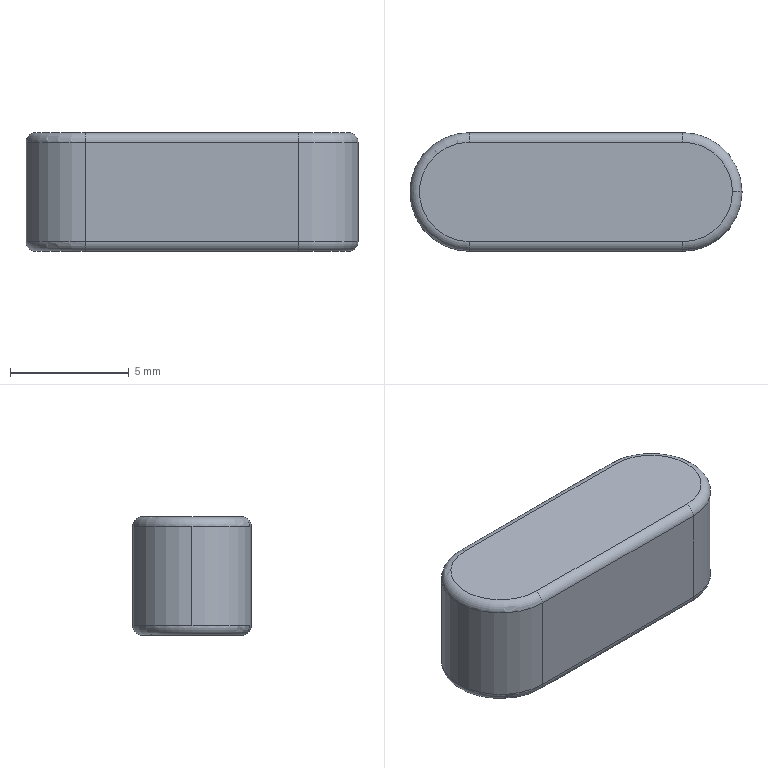Part | SolidWorks | features Extrusion 1, Fillet 1 | 1 solid | 17 faces | box 14 x 5 x 5 mm | volume 320.899 mm3 | cylinder 7 | torus 6 | plane 4 | commonest cylinder face diameters 0.8 x4 5 x3
STEP:
#1=CARTESIAN_POINT('',(6.6,0.,0.));
#2=VERTEX_POINT('',#1);
#3=CARTESIAN_POINT('',(4.5,-2.1,0.));
#4=VERTEX_POINT('',#3);
#5=CARTESIAN_POINT('',(4.5,0.,0.));
#6=DIRECTION('',(0.,0.,-1.));
#7=DIRECTION('',(1.,0.,0.));
#8=AXIS2_PLACEMENT_3D('',#5,#6,#7);
#9=CIRCLE('',#8,2.1);
#10=EDGE_CURVE('',#2,#4,#9,.T.);
#11=ORIENTED_EDGE('',*,*,#10,.F.);
#12=CARTESIAN_POINT('',(7.,0.,0.4));
#13=VERTEX_POINT('',#12);
#14=CARTESIAN_POINT('',(6.6,0.,0.4));
#15=DIRECTION('',(0.,-1.,0.));
#16=DIRECTION('',(0.,0.,-1.));
#17=AXIS2_PLACEMENT_3D('',#14,#15,#16);
#18=CIRCLE('',#17,0.4);
#19=EDGE_CURVE('',#2,#13,#18,.T.);
#20=ORIENTED_EDGE('',*,*,#19,.T.);
#21=CARTESIAN_POINT('',(4.5,-2.5,0.4));
#22=VERTEX_POINT('',#21);
#23=CARTESIAN_POINT('',(4.5,0.,0.4));
#24=DIRECTION('',(0.,0.,1.));
#25=DIRECTION('',(1.,0.,0.));
#26=AXIS2_PLACEMENT_3D('',#23,#24,#25);
#27=CIRCLE('',#26,2.5);
#28=EDGE_CURVE('',#22,#13,#27,.T.);
#29=ORIENTED_EDGE('',*,*,#28,.F.);
#30=CARTESIAN_POINT('',(4.5,-2.1,0.4));
#31=DIRECTION('',(1.,0.,0.));
#32=DIRECTION('',(0.,0.,-1.));
#33=AXIS2_PLACEMENT_3D('',#30,#31,#32);
#34=CIRCLE('',#33,0.4);
#35=EDGE_CURVE('',#22,#4,#34,.T.);
#36=ORIENTED_EDGE('',*,*,#35,.T.);
#37=EDGE_LOOP('',(#11,#20,#29,#36));
#38=FACE_OUTER_BOUND('',#37,.T.);
#39=CARTESIAN_POINT('',(4.5,0.,0.4));
#40=DIRECTION('',(0.,0.,1.));
#41=DIRECTION('',(1.,0.,0.));
#42=AXIS2_PLACEMENT_3D('',#39,#40,#41);
#43=TOROIDAL_SURFACE('',#42,2.1,0.4);
#44=ADVANCED_FACE('',(#38),#43,.T.);
#45=CARTESIAN_POINT('',(7.,0.,4.6));
#46=VERTEX_POINT('',#45);
#47=CARTESIAN_POINT('',(4.5,-2.5,4.6));
#48=VERTEX_POINT('',#47);
#49=CARTESIAN_POINT('',(4.5,0.,4.6));
#50=DIRECTION('',(0.,0.,-1.));
#51=DIRECTION('',(1.,0.,0.));
#52=AXIS2_PLACEMENT_3D('',#49,#50,#51);
#53=CIRCLE('',#52,2.5);
#54=EDGE_CURVE('',#46,#48,#53,.T.);
#55=ORIENTED_EDGE('',*,*,#54,.F.);
#56=CARTESIAN_POINT('',(6.6,0.,5.));
#57=VERTEX_POINT('',#56);
#58=CARTESIAN_POINT('',(6.6,0.,4.6));
#59=DIRECTION('',(0.,-1.,0.));
#60=DIRECTION('',(0.,0.,-1.));
#61=AXIS2_PLACEMENT_3D('',#58,#59,#60);
#62=CIRCLE('',#61,0.4);
#63=EDGE_CURVE('',#46,#57,#62,.T.);
#64=ORIENTED_EDGE('',*,*,#63,.T.);
#65=CARTESIAN_POINT('',(4.5,-2.1,5.));
#66=VERTEX_POINT('',#65);
#67=CARTESIAN_POINT('',(4.5,0.,5.));
#68=DIRECTION('',(0.,0.,1.));
#69=DIRECTION('',(1.,0.,0.));
#70=AXIS2_PLACEMENT_3D('',#67,#68,#69);
#71=CIRCLE('',#70,2.1);
#72=EDGE_CURVE('',#66,#57,#71,.T.);
#73=ORIENTED_EDGE('',*,*,#72,.F.);
#74=CARTESIAN_POINT('',(4.5,-2.1,4.6));
#75=DIRECTION('',(1.,0.,0.));
#76=DIRECTION('',(0.,0.,-1.));
#77=AXIS2_PLACEMENT_3D('',#74,#75,#76);
#78=CIRCLE('',#77,0.4);
#79=EDGE_CURVE('',#66,#48,#78,.T.);
#80=ORIENTED_EDGE('',*,*,#79,.T.);
#81=EDGE_LOOP('',(#55,#64,#73,#80));
#82=FACE_OUTER_BOUND('',#81,.T.);
#83=CARTESIAN_POINT('',(4.5,0.,4.6));
#84=DIRECTION('',(0.,0.,1.));
#85=DIRECTION('',(1.,0.,0.));
#86=AXIS2_PLACEMENT_3D('',#83,#84,#85);
#87=TOROIDAL_SURFACE('',#86,2.1,0.4);
#88=ADVANCED_FACE('',(#82),#87,.T.);
#89=CARTESIAN_POINT('',(-4.5,-2.5,4.6));
#90=VERTEX_POINT('',#89);
#91=CARTESIAN_POINT('',(-7.,0.,4.6));
#92=VERTEX_POINT('',#91);
#93=CARTESIAN_POINT('',(-4.5,0.,4.6));
#94=DIRECTION('',(0.,0.,-1.));
#95=DIRECTION('',(1.,0.,0.));
#96=AXIS2_PLACEMENT_3D('',#93,#94,#95);
#97=CIRCLE('',#96,2.5);
#98=EDGE_CURVE('',#90,#92,#97,.T.);
#99=ORIENTED_EDGE('',*,*,#98,.T.);
#100=CARTESIAN_POINT('',(-7.,0.,0.4));
#101=VERTEX_POINT('',#100);
#102=CARTESIAN_POINT('',(-7.,0.,5.));
#103=DIRECTION('',(0.,0.,-1.));
#104=VECTOR('',#103,1000.);
#105=LINE('',#102,#104);
#106=EDGE_CURVE('',#92,#101,#105,.T.);
#107=ORIENTED_EDGE('',*,*,#106,.T.);
#108=CARTESIAN_POINT('',(-4.5,-2.5,0.4));
#109=VERTEX_POINT('',#108);
#110=CARTESIAN_POINT('',(-4.5,0.,0.4));
#111=DIRECTION('',(0.,0.,1.));
#112=DIRECTION('',(1.,0.,0.));
#113=AXIS2_PLACEMENT_3D('',#110,#111,#112);
#114=CIRCLE('',#113,2.5);
#115=EDGE_CURVE('',#101,#109,#114,.T.);
#116=ORIENTED_EDGE('',*,*,#115,.T.);
#117=CARTESIAN_POINT('',(-4.5,-2.5,5.));
#118=DIRECTION('',(0.,0.,-1.));
#119=VECTOR('',#118,1000.);
#120=LINE('',#117,#119);
#121=EDGE_CURVE('',#90,#109,#120,.T.);
#122=ORIENTED_EDGE('',*,*,#121,.F.);
#123=EDGE_LOOP('',(#99,#107,#116,#122));
#124=FACE_OUTER_BOUND('',#123,.T.);
#125=CARTESIAN_POINT('',(-4.5,0.,5.));
#126=DIRECTION('',(0.,0.,-1.));
#127=DIRECTION('',(-1.,0.,0.));
#128=AXIS2_PLACEMENT_3D('',#125,#126,#127);
#129=CYLINDRICAL_SURFACE('',#128,2.5);
#130=ADVANCED_FACE('',(#124),#129,.T.);
#131=ORIENTED_EDGE('',*,*,#106,.F.);
#132=CARTESIAN_POINT('',(-4.5,2.5,4.6));
#133=VERTEX_POINT('',#132);
#134=CARTESIAN_POINT('',(-4.5,0.,4.6));
#135=DIRECTION('',(0.,0.,-1.));
#136=DIRECTION('',(1.,0.,0.));
#137=AXIS2_PLACEMENT_3D('',#134,#135,#136);
#138=CIRCLE('',#137,2.5);
#139=EDGE_CURVE('',#92,#133,#138,.T.);
#140=ORIENTED_EDGE('',*,*,#139,.T.);
#141=CARTESIAN_POINT('',(-4.5,2.5,0.4));
#142=VERTEX_POINT('',#141);
#143=CARTESIAN_POINT('',(-4.5,2.5,5.));
#144=DIRECTION('',(0.,0.,-1.));
#145=VECTOR('',#144,1000.);
#146=LINE('',#143,#145);
#147=EDGE_CURVE('',#133,#142,#146,.T.);
#148=ORIENTED_EDGE('',*,*,#147,.T.);
#149=CARTESIAN_POINT('',(-4.5,0.,0.4));
#150=DIRECTION('',(0.,0.,1.));
#151=DIRECTION('',(1.,0.,0.));
#152=AXIS2_PLACEMENT_3D('',#149,#150,#151);
#153=CIRCLE('',#152,2.5);
#154=EDGE_CURVE('',#142,#101,#153,.T.);
#155=ORIENTED_EDGE('',*,*,#154,.T.);
#156=EDGE_LOOP('',(#131,#140,#148,#155));
#157=FACE_OUTER_BOUND('',#156,.T.);
#158=CARTESIAN_POINT('',(-4.5,0.,5.));
#159=DIRECTION('',(0.,0.,-1.));
#160=DIRECTION('',(-1.,0.,0.));
#161=AXIS2_PLACEMENT_3D('',#158,#159,#160);
#162=CYLINDRICAL_SURFACE('',#161,2.5);
#163=ADVANCED_FACE('',(#157),#162,.T.);
#164=CARTESIAN_POINT('',(4.5,-2.5,5.));
#165=DIRECTION('',(0.,0.,-1.));
#166=VECTOR('',#165,1000.);
#167=LINE('',#164,#166);
#168=EDGE_CURVE('',#48,#22,#167,.T.);
#169=ORIENTED_EDGE('',*,*,#168,.F.);
#170=CARTESIAN_POINT('',(-4.5,-2.5,4.6));
#171=DIRECTION('',(-1.,0.,0.));
#172=VECTOR('',#171,1000.);
#173=LINE('',#170,#172);
#174=EDGE_CURVE('',#48,#90,#173,.T.);
#175=ORIENTED_EDGE('',*,*,#174,.T.);
#176=ORIENTED_EDGE('',*,*,#121,.T.);
#177=CARTESIAN_POINT('',(-4.5,-2.5,0.4));
#178=DIRECTION('',(1.,0.,0.));
#179=VECTOR('',#178,1000.);
#180=LINE('',#177,#179);
#181=EDGE_CURVE('',#109,#22,#180,.T.);
#182=ORIENTED_EDGE('',*,*,#181,.T.);
#183=EDGE_LOOP('',(#169,#175,#176,#182));
#184=FACE_OUTER_BOUND('',#183,.T.);
#185=CARTESIAN_POINT('',(-4.5,-2.5,5.));
#186=DIRECTION('',(0.,1.,0.));
#187=DIRECTION('',(-1.,0.,0.));
#188=AXIS2_PLACEMENT_3D('',#185,#186,#187);
#189=PLANE('',#188);
#190=ADVANCED_FACE('',(#184),#189,.F.);
#191=CARTESIAN_POINT('',(4.5,2.5,4.6));
#192=VERTEX_POINT('',#191);
#193=CARTESIAN_POINT('',(4.5,2.5,0.4));
#194=VERTEX_POINT('',#193);
#195=CARTESIAN_POINT('',(4.5,2.5,5.));
#196=DIRECTION('',(0.,0.,-1.));
#197=VECTOR('',#196,1000.);
#198=LINE('',#195,#197);
#199=EDGE_CURVE('',#192,#194,#198,.T.);
#200=ORIENTED_EDGE('',*,*,#199,.F.);
#201=CARTESIAN_POINT('',(4.5,0.,4.6));
#202=DIRECTION('',(0.,0.,-1.));
#203=DIRECTION('',(1.,0.,0.));
#204=AXIS2_PLACEMENT_3D('',#201,#202,#203);
#205=CIRCLE('',#204,2.5);
#206=EDGE_CURVE('',#192,#46,#205,.T.);
#207=ORIENTED_EDGE('',*,*,#206,.T.);
#208=ORIENTED_EDGE('',*,*,#54,.T.);
#209=ORIENTED_EDGE('',*,*,#168,.T.);
#210=ORIENTED_EDGE('',*,*,#28,.T.);
#211=CARTESIAN_POINT('',(4.5,0.,0.4));
#212=DIRECTION('',(0.,0.,1.));
#213=DIRECTION('',(1.,0.,0.));
#214=AXIS2_PLACEMENT_3D('',#211,#212,#213);
#215=CIRCLE('',#214,2.5);
#216=EDGE_CURVE('',#13,#194,#215,.T.);
#217=ORIENTED_EDGE('',*,*,#216,.T.);
#218=EDGE_LOOP('',(#200,#207,#208,#209,#210,#217));
#219=FACE_OUTER_BOUND('',#218,.T.);
#220=CARTESIAN_POINT('',(4.5,0.,5.));
#221=DIRECTION('',(0.,0.,-1.));
#222=DIRECTION('',(-1.,0.,0.));
#223=AXIS2_PLACEMENT_3D('',#220,#221,#222);
#224=CYLINDRICAL_SURFACE('',#223,2.5);
#225=ADVANCED_FACE('',(#219),#224,.T.);
#226=ORIENTED_EDGE('',*,*,#147,.F.);
#227=CARTESIAN_POINT('',(4.5,2.5,4.6));
#228=DIRECTION('',(1.,0.,0.));
#229=VECTOR('',#228,1000.);
#230=LINE('',#227,#229);
#231=EDGE_CURVE('',#133,#192,#230,.T.);
#232=ORIENTED_EDGE('',*,*,#231,.T.);
#233=ORIENTED_EDGE('',*,*,#199,.T.);
#234=CARTESIAN_POINT('',(-4.5,2.5,0.4));
#235=DIRECTION('',(-1.,0.,0.));
#236=VECTOR('',#235,1000.);
#237=LINE('',#234,#236);
#238=EDGE_CURVE('',#194,#142,#237,.T.);
#239=ORIENTED_EDGE('',*,*,#238,.T.);
#240=EDGE_LOOP('',(#226,#232,#233,#239));
#241=FACE_OUTER_BOUND('',#240,.T.);
#242=CARTESIAN_POINT('',(-4.5,2.5,5.));
#243=DIRECTION('',(0.,-1.,0.));
#244=DIRECTION('',(1.,0.,0.));
#245=AXIS2_PLACEMENT_3D('',#242,#243,#244);
#246=PLANE('',#245);
#247=ADVANCED_FACE('',(#241),#246,.F.);
#248=CARTESIAN_POINT('',(-4.5,-2.1,5.));
#249=VERTEX_POINT('',#248);
#250=CARTESIAN_POINT('',(4.5,-2.1,5.));
#251=DIRECTION('',(1.,0.,0.));
#252=VECTOR('',#251,1000.);
#253=LINE('',#250,#252);
#254=EDGE_CURVE('',#249,#66,#253,.T.);
#255=ORIENTED_EDGE('',*,*,#254,.T.);
#256=ORIENTED_EDGE('',*,*,#72,.T.);
#257=CARTESIAN_POINT('',(4.5,2.1,5.));
#258=VERTEX_POINT('',#257);
#259=CARTESIAN_POINT('',(4.5,0.,5.));
#260=DIRECTION('',(0.,0.,1.));
#261=DIRECTION('',(1.,0.,0.));
#262=AXIS2_PLACEMENT_3D('',#259,#260,#261);
#263=CIRCLE('',#262,2.1);
#264=EDGE_CURVE('',#57,#258,#263,.T.);
#265=ORIENTED_EDGE('',*,*,#264,.T.);
#266=CARTESIAN_POINT('',(-4.5,2.1,5.));
#267=VERTEX_POINT('',#266);
#268=CARTESIAN_POINT('',(-4.5,2.1,5.));
#269=DIRECTION('',(-1.,0.,0.));
#270=VECTOR('',#269,1000.);
#271=LINE('',#268,#270);
#272=EDGE_CURVE('',#258,#267,#271,.T.);
#273=ORIENTED_EDGE('',*,*,#272,.T.);
#274=CARTESIAN_POINT('',(-4.5,0.,5.));
#275=DIRECTION('',(0.,0.,1.));
#276=DIRECTION('',(1.,0.,0.));
#277=AXIS2_PLACEMENT_3D('',#274,#275,#276);
#278=CIRCLE('',#277,2.1);
#279=EDGE_CURVE('',#267,#249,#278,.T.);
#280=ORIENTED_EDGE('',*,*,#279,.T.);
#281=EDGE_LOOP('',(#255,#256,#265,#273,#280));
#282=FACE_OUTER_BOUND('',#281,.T.);
#283=CARTESIAN_POINT('',(-4.5,0.,5.));
#284=DIRECTION('',(0.,0.,1.));
#285=DIRECTION('',(1.,0.,0.));
#286=AXIS2_PLACEMENT_3D('',#283,#284,#285);
#287=PLANE('',#286);
#288=ADVANCED_FACE('',(#282),#287,.T.);
#289=CARTESIAN_POINT('',(-4.5,2.1,0.));
#290=VERTEX_POINT('',#289);
#291=CARTESIAN_POINT('',(4.5,2.1,0.));
#292=VERTEX_POINT('',#291);
#293=CARTESIAN_POINT('',(-4.5,2.1,0.));
#294=DIRECTION('',(1.,0.,0.));
#295=VECTOR('',#294,1000.);
#296=LINE('',#293,#295);
#297=EDGE_CURVE('',#290,#292,#296,.T.);
#298=ORIENTED_EDGE('',*,*,#297,.T.);
#299=CARTESIAN_POINT('',(4.5,0.,0.));
#300=DIRECTION('',(0.,0.,-1.));
#301=DIRECTION('',(1.,0.,0.));
#302=AXIS2_PLACEMENT_3D('',#299,#300,#301);
#303=CIRCLE('',#302,2.1);
#304=EDGE_CURVE('',#292,#2,#303,.T.);
#305=ORIENTED_EDGE('',*,*,#304,.T.);
#306=ORIENTED_EDGE('',*,*,#10,.T.);
#307=CARTESIAN_POINT('',(-4.5,-2.1,0.));
#308=VERTEX_POINT('',#307);
#309=CARTESIAN_POINT('',(-4.5,-2.1,0.));
#310=DIRECTION('',(-1.,0.,0.));
#311=VECTOR('',#310,1000.);
#312=LINE('',#309,#311);
#313=EDGE_CURVE('',#4,#308,#312,.T.);
#314=ORIENTED_EDGE('',*,*,#313,.T.);
#315=CARTESIAN_POINT('',(-4.5,0.,0.));
#316=DIRECTION('',(0.,0.,-1.));
#317=DIRECTION('',(1.,0.,0.));
#318=AXIS2_PLACEMENT_3D('',#315,#316,#317);
#319=CIRCLE('',#318,2.1);
#320=EDGE_CURVE('',#308,#290,#319,.T.);
#321=ORIENTED_EDGE('',*,*,#320,.T.);
#322=EDGE_LOOP('',(#298,#305,#306,#314,#321));
#323=FACE_OUTER_BOUND('',#322,.T.);
#324=CARTESIAN_POINT('',(-4.5,0.,0.));
#325=DIRECTION('',(0.,0.,1.));
#326=DIRECTION('',(1.,0.,0.));
#327=AXIS2_PLACEMENT_3D('',#324,#325,#326);
#328=PLANE('',#327);
#329=ADVANCED_FACE('',(#323),#328,.F.);
#330=CARTESIAN_POINT('',(-4.5,2.1,4.6));
#331=DIRECTION('',(1.,0.,0.));
#332=DIRECTION('',(0.,0.,-1.));
#333=AXIS2_PLACEMENT_3D('',#330,#331,#332);
#334=CIRCLE('',#333,0.4);
#335=EDGE_CURVE('',#133,#267,#334,.T.);
#336=ORIENTED_EDGE('',*,*,#335,.F.);
#337=ORIENTED_EDGE('',*,*,#139,.F.);
#338=ORIENTED_EDGE('',*,*,#98,.F.);
#339=CARTESIAN_POINT('',(-4.5,-2.1,4.6));
#340=DIRECTION('',(1.,0.,0.));
#341=DIRECTION('',(0.,0.,-1.));
#342=AXIS2_PLACEMENT_3D('',#339,#340,#341);
#343=CIRCLE('',#342,0.4);
#344=EDGE_CURVE('',#249,#90,#343,.T.);
#345=ORIENTED_EDGE('',*,*,#344,.F.);
#346=ORIENTED_EDGE('',*,*,#279,.F.);
#347=EDGE_LOOP('',(#336,#337,#338,#345,#346));
#348=FACE_OUTER_BOUND('',#347,.T.);
#349=CARTESIAN_POINT('',(-4.5,0.,4.6));
#350=DIRECTION('',(0.,0.,1.));
#351=DIRECTION('',(1.,0.,0.));
#352=AXIS2_PLACEMENT_3D('',#349,#350,#351);
#353=TOROIDAL_SURFACE('',#352,2.1,0.4);
#354=ADVANCED_FACE('',(#348),#353,.T.);
#355=ORIENTED_EDGE('',*,*,#344,.T.);
#356=ORIENTED_EDGE('',*,*,#174,.F.);
#357=ORIENTED_EDGE('',*,*,#79,.F.);
#358=ORIENTED_EDGE('',*,*,#254,.F.);
#359=EDGE_LOOP('',(#355,#356,#357,#358));
#360=FACE_OUTER_BOUND('',#359,.T.);
#361=CARTESIAN_POINT('',(-4.5,-2.1,4.6));
#362=DIRECTION('',(-1.,0.,0.));
#363=DIRECTION('',(0.,-1.,0.));
#364=AXIS2_PLACEMENT_3D('',#361,#362,#363);
#365=CYLINDRICAL_SURFACE('',#364,0.4);
#366=ADVANCED_FACE('',(#360),#365,.T.);
#367=ORIENTED_EDGE('',*,*,#335,.T.);
#368=ORIENTED_EDGE('',*,*,#272,.F.);
#369=CARTESIAN_POINT('',(4.5,2.1,4.6));
#370=DIRECTION('',(1.,0.,0.));
#371=DIRECTION('',(0.,0.,-1.));
#372=AXIS2_PLACEMENT_3D('',#369,#370,#371);
#373=CIRCLE('',#372,0.4);
#374=EDGE_CURVE('',#192,#258,#373,.T.);
#375=ORIENTED_EDGE('',*,*,#374,.F.);
#376=ORIENTED_EDGE('',*,*,#231,.F.);
#377=EDGE_LOOP('',(#367,#368,#375,#376));
#378=FACE_OUTER_BOUND('',#377,.T.);
#379=CARTESIAN_POINT('',(-4.5,2.1,4.6));
#380=DIRECTION('',(1.,0.,0.));
#381=DIRECTION('',(0.,1.,0.));
#382=AXIS2_PLACEMENT_3D('',#379,#380,#381);
#383=CYLINDRICAL_SURFACE('',#382,0.4);
#384=ADVANCED_FACE('',(#378),#383,.T.);
#385=ORIENTED_EDGE('',*,*,#63,.F.);
#386=ORIENTED_EDGE('',*,*,#206,.F.);
#387=ORIENTED_EDGE('',*,*,#374,.T.);
#388=ORIENTED_EDGE('',*,*,#264,.F.);
#389=EDGE_LOOP('',(#385,#386,#387,#388));
#390=FACE_OUTER_BOUND('',#389,.T.);
#391=CARTESIAN_POINT('',(4.5,0.,4.6));
#392=DIRECTION('',(0.,0.,1.));
#393=DIRECTION('',(1.,0.,0.));
#394=AXIS2_PLACEMENT_3D('',#391,#392,#393);
#395=TOROIDAL_SURFACE('',#394,2.1,0.4);
#396=ADVANCED_FACE('',(#390),#395,.T.);
#397=CARTESIAN_POINT('',(-4.5,2.1,0.4));
#398=DIRECTION('',(1.,0.,0.));
#399=DIRECTION('',(0.,0.,-1.));
#400=AXIS2_PLACEMENT_3D('',#397,#398,#399);
#401=CIRCLE('',#400,0.4);
#402=EDGE_CURVE('',#290,#142,#401,.T.);
#403=ORIENTED_EDGE('',*,*,#402,.F.);
#404=ORIENTED_EDGE('',*,*,#320,.F.);
#405=CARTESIAN_POINT('',(-4.5,-2.1,0.4));
#406=DIRECTION('',(1.,0.,0.));
#407=DIRECTION('',(0.,0.,-1.));
#408=AXIS2_PLACEMENT_3D('',#405,#406,#407);
#409=CIRCLE('',#408,0.4);
#410=EDGE_CURVE('',#109,#308,#409,.T.);
#411=ORIENTED_EDGE('',*,*,#410,.F.);
#412=ORIENTED_EDGE('',*,*,#115,.F.);
#413=ORIENTED_EDGE('',*,*,#154,.F.);
#414=EDGE_LOOP('',(#403,#404,#411,#412,#413));
#415=FACE_OUTER_BOUND('',#414,.T.);
#416=CARTESIAN_POINT('',(-4.5,0.,0.4));
#417=DIRECTION('',(0.,0.,1.));
#418=DIRECTION('',(1.,0.,0.));
#419=AXIS2_PLACEMENT_3D('',#416,#417,#418);
#420=TOROIDAL_SURFACE('',#419,2.1,0.4);
#421=ADVANCED_FACE('',(#415),#420,.T.);
#422=ORIENTED_EDGE('',*,*,#410,.T.);
#423=ORIENTED_EDGE('',*,*,#313,.F.);
#424=ORIENTED_EDGE('',*,*,#35,.F.);
#425=ORIENTED_EDGE('',*,*,#181,.F.);
#426=EDGE_LOOP('',(#422,#423,#424,#425));
#427=FACE_OUTER_BOUND('',#426,.T.);
#428=CARTESIAN_POINT('',(-4.5,-2.1,0.4));
#429=DIRECTION('',(1.,0.,0.));
#430=DIRECTION('',(0.,1.,0.));
#431=AXIS2_PLACEMENT_3D('',#428,#429,#430);
#432=CYLINDRICAL_SURFACE('',#431,0.4);
#433=ADVANCED_FACE('',(#427),#432,.T.);
#434=ORIENTED_EDGE('',*,*,#402,.T.);
#435=ORIENTED_EDGE('',*,*,#238,.F.);
#436=CARTESIAN_POINT('',(4.5,2.1,0.4));
#437=DIRECTION('',(1.,0.,0.));
#438=DIRECTION('',(0.,0.,-1.));
#439=AXIS2_PLACEMENT_3D('',#436,#437,#438);
#440=CIRCLE('',#439,0.4);
#441=EDGE_CURVE('',#292,#194,#440,.T.);
#442=ORIENTED_EDGE('',*,*,#441,.F.);
#443=ORIENTED_EDGE('',*,*,#297,.F.);
#444=EDGE_LOOP('',(#434,#435,#442,#443));
#445=FACE_OUTER_BOUND('',#444,.T.);
#446=CARTESIAN_POINT('',(-4.5,2.1,0.4));
#447=DIRECTION('',(-1.,0.,0.));
#448=DIRECTION('',(0.,-1.,0.));
#449=AXIS2_PLACEMENT_3D('',#446,#447,#448);
#450=CYLINDRICAL_SURFACE('',#449,0.4);
#451=ADVANCED_FACE('',(#445),#450,.T.);
#452=ORIENTED_EDGE('',*,*,#19,.F.);
#453=ORIENTED_EDGE('',*,*,#304,.F.);
#454=ORIENTED_EDGE('',*,*,#441,.T.);
#455=ORIENTED_EDGE('',*,*,#216,.F.);
#456=EDGE_LOOP('',(#452,#453,#454,#455));
#457=FACE_OUTER_BOUND('',#456,.T.);
#458=CARTESIAN_POINT('',(4.5,0.,0.4));
#459=DIRECTION('',(0.,0.,1.));
#460=DIRECTION('',(1.,0.,0.));
#461=AXIS2_PLACEMENT_3D('',#458,#459,#460);
#462=TOROIDAL_SURFACE('',#461,2.1,0.4);
#463=ADVANCED_FACE('',(#457),#462,.T.);
#464=CLOSED_SHELL('',(#44,#88,#130,#163,#190,#225,#247,#288,#329,#354,#366,#384,#396,#421,#433,#451,#463));
#465=MANIFOLD_SOLID_BREP('',#464);
#466=CARTESIAN_POINT('',(0.,0.,0.));
#467=DIRECTION('',(0.,0.,1.));
#468=DIRECTION('',(1.,0.,0.));
#469=AXIS2_PLACEMENT_3D('',#466,#467,#468);
#470=(LENGTH_UNIT()NAMED_UNIT(*)SI_UNIT(.MILLI.,.METRE.));
#471=UNCERTAINTY_MEASURE_WITH_UNIT(LENGTH_MEASURE(0.00001),#470,'','');
#472=(NAMED_UNIT(*)PLANE_ANGLE_UNIT()SI_UNIT($,.RADIAN.));
#473=(NAMED_UNIT(*)SI_UNIT($,.STERADIAN.)SOLID_ANGLE_UNIT());
#474=(GEOMETRIC_REPRESENTATION_CONTEXT(3)GLOBAL_UNCERTAINTY_ASSIGNED_CONTEXT((#471))GLOBAL_UNIT_ASSIGNED_CONTEXT((#470,#472,#473))REPRESENTATION_CONTEXT('',''));
#475=ADVANCED_BREP_SHAPE_REPRESENTATION('',(#465,#469),#474);